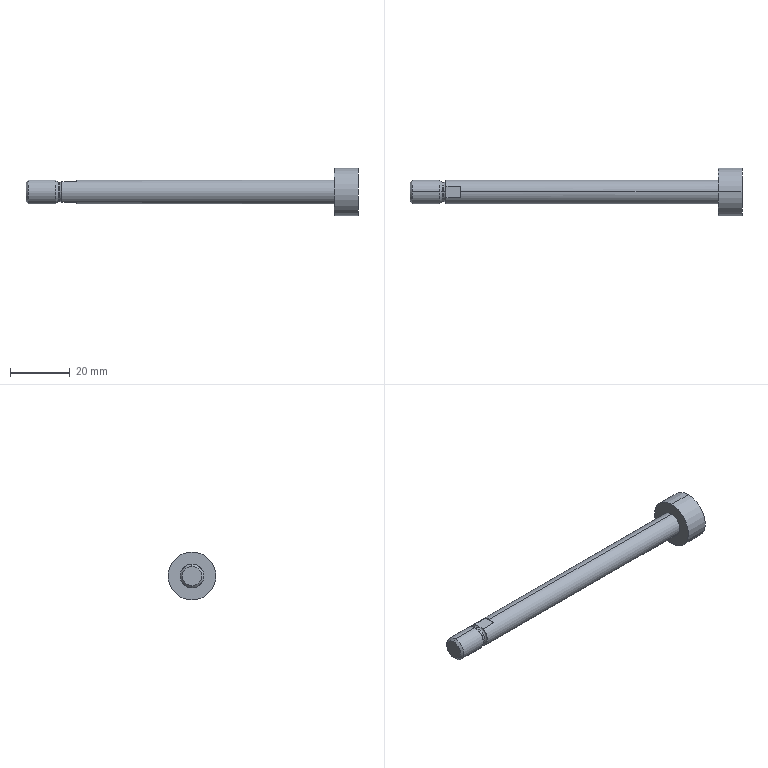Part | STEP file | 9123_DGS_16_10_P_k_HI | 1 solid | 23 faces | box 111 x 16 x 16 mm | volume 6739 mm3 | plane 9 | cylinder 8 | cone 4 | torus 2 | commonest cylinder face diameters 8 x4 6.466 x2 16 x2